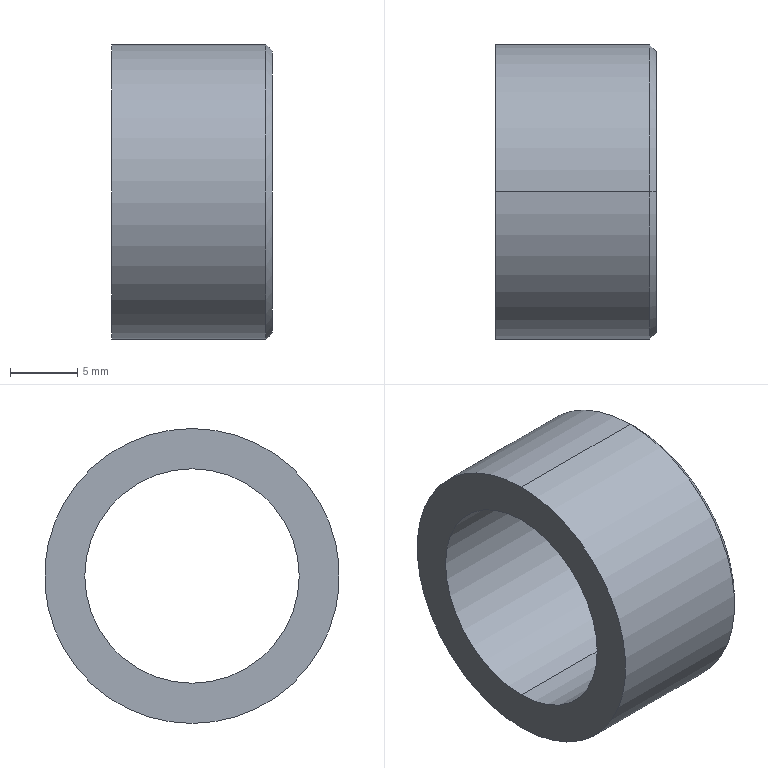Part | STEP file | Guide wheel mechanism revised.sldasm-Part-41 | 1 solid | 10 faces | box 12 x 22 x 22 mm | volume 2134 mm3 | cone 4 | cylinder 4 | plane 2 | commonest cylinder face diameters 16 x2 22 x2
STEP:
#1=CARTESIAN_POINT('',(11.5,0.,8.));
#2=VERTEX_POINT('',#1);
#3=CARTESIAN_POINT('',(11.5,0.,-8.));
#4=VERTEX_POINT('',#3);
#5=CARTESIAN_POINT('',(11.5,0.,0.));
#6=DIRECTION('',(1.,0.,0.));
#7=DIRECTION('',(0.,0.,1.));
#8=AXIS2_PLACEMENT_3D('',#5,#6,#7);
#9=CIRCLE('',#8,8.);
#10=EDGE_CURVE('',#2,#4,#9,.T.);
#11=ORIENTED_EDGE('',*,*,#10,.F.);
#12=CARTESIAN_POINT('',(12.,0.,8.5));
#13=VERTEX_POINT('',#12);
#14=CARTESIAN_POINT('',(12.,0.,8.5));
#15=DIRECTION('',(0.7071,0.,0.7071));
#16=VECTOR('',#15,1000.);
#17=LINE('',#14,#16);
#18=EDGE_CURVE('',#2,#13,#17,.T.);
#19=ORIENTED_EDGE('',*,*,#18,.T.);
#20=CARTESIAN_POINT('',(12.,0.,-8.5));
#21=VERTEX_POINT('',#20);
#22=CARTESIAN_POINT('',(12.,0.,0.));
#23=DIRECTION('',(-1.,0.,0.));
#24=DIRECTION('',(0.,0.,1.));
#25=AXIS2_PLACEMENT_3D('',#22,#23,#24);
#26=CIRCLE('',#25,8.5);
#27=EDGE_CURVE('',#21,#13,#26,.T.);
#28=ORIENTED_EDGE('',*,*,#27,.F.);
#29=CARTESIAN_POINT('',(12.,0.,-8.5));
#30=DIRECTION('',(0.7071,0.,-0.7071));
#31=VECTOR('',#30,1000.);
#32=LINE('',#29,#31);
#33=EDGE_CURVE('',#4,#21,#32,.T.);
#34=ORIENTED_EDGE('',*,*,#33,.F.);
#35=EDGE_LOOP('',(#11,#19,#28,#34));
#36=FACE_OUTER_BOUND('',#35,.T.);
#37=CARTESIAN_POINT('',(12.,0.,0.));
#38=DIRECTION('',(1.,0.,0.));
#39=DIRECTION('',(0.,0.,-1.));
#40=AXIS2_PLACEMENT_3D('',#37,#38,#39);
#41=CONICAL_SURFACE('',#40,8.5,0.7854);
#42=ADVANCED_FACE('',(#36),#41,.F.);
#43=CARTESIAN_POINT('',(12.,0.,-10.5));
#44=VERTEX_POINT('',#43);
#45=CARTESIAN_POINT('',(12.,0.,10.5));
#46=VERTEX_POINT('',#45);
#47=CARTESIAN_POINT('',(12.,0.,0.));
#48=DIRECTION('',(1.,0.,0.));
#49=DIRECTION('',(0.,0.,1.));
#50=AXIS2_PLACEMENT_3D('',#47,#48,#49);
#51=CIRCLE('',#50,10.5);
#52=EDGE_CURVE('',#44,#46,#51,.T.);
#53=ORIENTED_EDGE('',*,*,#52,.F.);
#54=CARTESIAN_POINT('',(11.5,0.,-11.));
#55=VERTEX_POINT('',#54);
#56=CARTESIAN_POINT('',(11.5,0.,-11.));
#57=DIRECTION('',(-0.7071,0.,-0.7071));
#58=VECTOR('',#57,1000.);
#59=LINE('',#56,#58);
#60=EDGE_CURVE('',#44,#55,#59,.T.);
#61=ORIENTED_EDGE('',*,*,#60,.T.);
#62=CARTESIAN_POINT('',(11.5,0.,11.));
#63=VERTEX_POINT('',#62);
#64=CARTESIAN_POINT('',(11.5,0.,0.));
#65=DIRECTION('',(-1.,0.,0.));
#66=DIRECTION('',(0.,0.,1.));
#67=AXIS2_PLACEMENT_3D('',#64,#65,#66);
#68=CIRCLE('',#67,11.);
#69=EDGE_CURVE('',#63,#55,#68,.T.);
#70=ORIENTED_EDGE('',*,*,#69,.F.);
#71=CARTESIAN_POINT('',(11.5,0.,11.));
#72=DIRECTION('',(-0.7071,0.,0.7071));
#73=VECTOR('',#72,1000.);
#74=LINE('',#71,#73);
#75=EDGE_CURVE('',#46,#63,#74,.T.);
#76=ORIENTED_EDGE('',*,*,#75,.F.);
#77=EDGE_LOOP('',(#53,#61,#70,#76));
#78=FACE_OUTER_BOUND('',#77,.T.);
#79=CARTESIAN_POINT('',(11.5,0.,0.));
#80=DIRECTION('',(-1.,0.,0.));
#81=DIRECTION('',(0.,0.,1.));
#82=AXIS2_PLACEMENT_3D('',#79,#80,#81);
#83=CONICAL_SURFACE('',#82,11.,0.7854);
#84=ADVANCED_FACE('',(#78),#83,.T.);
#85=ORIENTED_EDGE('',*,*,#69,.T.);
#86=CARTESIAN_POINT('',(0.,0.,-11.));
#87=VERTEX_POINT('',#86);
#88=CARTESIAN_POINT('',(12.,0.,-11.));
#89=DIRECTION('',(-1.,0.,0.));
#90=VECTOR('',#89,1000.);
#91=LINE('',#88,#90);
#92=EDGE_CURVE('',#55,#87,#91,.T.);
#93=ORIENTED_EDGE('',*,*,#92,.T.);
#94=CARTESIAN_POINT('',(0.,0.,11.));
#95=VERTEX_POINT('',#94);
#96=CARTESIAN_POINT('',(0.,0.,0.));
#97=DIRECTION('',(-1.,0.,0.));
#98=DIRECTION('',(0.,0.,1.));
#99=AXIS2_PLACEMENT_3D('',#96,#97,#98);
#100=CIRCLE('',#99,11.);
#101=EDGE_CURVE('',#95,#87,#100,.T.);
#102=ORIENTED_EDGE('',*,*,#101,.F.);
#103=CARTESIAN_POINT('',(12.,0.,11.));
#104=DIRECTION('',(-1.,0.,0.));
#105=VECTOR('',#104,1000.);
#106=LINE('',#103,#105);
#107=EDGE_CURVE('',#63,#95,#106,.T.);
#108=ORIENTED_EDGE('',*,*,#107,.F.);
#109=EDGE_LOOP('',(#85,#93,#102,#108));
#110=FACE_OUTER_BOUND('',#109,.T.);
#111=CARTESIAN_POINT('',(12.,0.,0.));
#112=DIRECTION('',(-1.,0.,0.));
#113=DIRECTION('',(0.,0.,1.));
#114=AXIS2_PLACEMENT_3D('',#111,#112,#113);
#115=CYLINDRICAL_SURFACE('',#114,11.);
#116=ADVANCED_FACE('',(#110),#115,.T.);
#117=ORIENTED_EDGE('',*,*,#10,.T.);
#118=CARTESIAN_POINT('',(0.,0.,-8.));
#119=VERTEX_POINT('',#118);
#120=CARTESIAN_POINT('',(12.,0.,-8.));
#121=DIRECTION('',(-1.,0.,0.));
#122=VECTOR('',#121,1000.);
#123=LINE('',#120,#122);
#124=EDGE_CURVE('',#4,#119,#123,.T.);
#125=ORIENTED_EDGE('',*,*,#124,.T.);
#126=CARTESIAN_POINT('',(0.,0.,8.));
#127=VERTEX_POINT('',#126);
#128=CARTESIAN_POINT('',(0.,0.,0.));
#129=DIRECTION('',(-1.,0.,0.));
#130=DIRECTION('',(0.,0.,1.));
#131=AXIS2_PLACEMENT_3D('',#128,#129,#130);
#132=CIRCLE('',#131,8.);
#133=EDGE_CURVE('',#119,#127,#132,.T.);
#134=ORIENTED_EDGE('',*,*,#133,.T.);
#135=CARTESIAN_POINT('',(12.,0.,8.));
#136=DIRECTION('',(-1.,0.,0.));
#137=VECTOR('',#136,1000.);
#138=LINE('',#135,#137);
#139=EDGE_CURVE('',#2,#127,#138,.T.);
#140=ORIENTED_EDGE('',*,*,#139,.F.);
#141=EDGE_LOOP('',(#117,#125,#134,#140));
#142=FACE_OUTER_BOUND('',#141,.T.);
#143=CARTESIAN_POINT('',(12.,0.,0.));
#144=DIRECTION('',(-1.,0.,0.));
#145=DIRECTION('',(0.,0.,1.));
#146=AXIS2_PLACEMENT_3D('',#143,#144,#145);
#147=CYLINDRICAL_SURFACE('',#146,8.);
#148=ADVANCED_FACE('',(#142),#147,.F.);
#149=ORIENTED_EDGE('',*,*,#124,.F.);
#150=CARTESIAN_POINT('',(11.5,0.,0.));
#151=DIRECTION('',(1.,0.,0.));
#152=DIRECTION('',(0.,0.,1.));
#153=AXIS2_PLACEMENT_3D('',#150,#151,#152);
#154=CIRCLE('',#153,8.);
#155=EDGE_CURVE('',#4,#2,#154,.T.);
#156=ORIENTED_EDGE('',*,*,#155,.T.);
#157=ORIENTED_EDGE('',*,*,#139,.T.);
#158=CARTESIAN_POINT('',(0.,0.,0.));
#159=DIRECTION('',(-1.,0.,0.));
#160=DIRECTION('',(0.,0.,1.));
#161=AXIS2_PLACEMENT_3D('',#158,#159,#160);
#162=CIRCLE('',#161,8.);
#163=EDGE_CURVE('',#127,#119,#162,.T.);
#164=ORIENTED_EDGE('',*,*,#163,.T.);
#165=EDGE_LOOP('',(#149,#156,#157,#164));
#166=FACE_OUTER_BOUND('',#165,.T.);
#167=CARTESIAN_POINT('',(12.,0.,0.));
#168=DIRECTION('',(-1.,0.,0.));
#169=DIRECTION('',(0.,0.,1.));
#170=AXIS2_PLACEMENT_3D('',#167,#168,#169);
#171=CYLINDRICAL_SURFACE('',#170,8.);
#172=ADVANCED_FACE('',(#166),#171,.F.);
#173=ORIENTED_EDGE('',*,*,#27,.T.);
#174=CARTESIAN_POINT('',(12.,0.,0.));
#175=DIRECTION('',(-1.,0.,0.));
#176=DIRECTION('',(0.,0.,1.));
#177=AXIS2_PLACEMENT_3D('',#174,#175,#176);
#178=CIRCLE('',#177,8.5);
#179=EDGE_CURVE('',#13,#21,#178,.T.);
#180=ORIENTED_EDGE('',*,*,#179,.T.);
#181=EDGE_LOOP('',(#173,#180));
#182=FACE_BOUND('',#181,.T.);
#183=CARTESIAN_POINT('',(12.,0.,0.));
#184=DIRECTION('',(1.,0.,0.));
#185=DIRECTION('',(0.,0.,1.));
#186=AXIS2_PLACEMENT_3D('',#183,#184,#185);
#187=CIRCLE('',#186,10.5);
#188=EDGE_CURVE('',#46,#44,#187,.T.);
#189=ORIENTED_EDGE('',*,*,#188,.T.);
#190=ORIENTED_EDGE('',*,*,#52,.T.);
#191=EDGE_LOOP('',(#189,#190));
#192=FACE_OUTER_BOUND('',#191,.T.);
#193=CARTESIAN_POINT('',(12.,9.,0.));
#194=DIRECTION('',(-1.,0.,0.));
#195=DIRECTION('',(0.,0.,1.));
#196=AXIS2_PLACEMENT_3D('',#193,#194,#195);
#197=PLANE('',#196);
#198=ADVANCED_FACE('',(#182,#192),#197,.F.);
#199=ORIENTED_EDGE('',*,*,#163,.F.);
#200=ORIENTED_EDGE('',*,*,#133,.F.);
#201=EDGE_LOOP('',(#199,#200));
#202=FACE_BOUND('',#201,.T.);
#203=ORIENTED_EDGE('',*,*,#101,.T.);
#204=CARTESIAN_POINT('',(0.,0.,0.));
#205=DIRECTION('',(-1.,0.,0.));
#206=DIRECTION('',(0.,0.,1.));
#207=AXIS2_PLACEMENT_3D('',#204,#205,#206);
#208=CIRCLE('',#207,11.);
#209=EDGE_CURVE('',#87,#95,#208,.T.);
#210=ORIENTED_EDGE('',*,*,#209,.T.);
#211=EDGE_LOOP('',(#203,#210));
#212=FACE_OUTER_BOUND('',#211,.T.);
#213=CARTESIAN_POINT('',(0.,10.,0.));
#214=DIRECTION('',(1.,0.,0.));
#215=DIRECTION('',(0.,0.,-1.));
#216=AXIS2_PLACEMENT_3D('',#213,#214,#215);
#217=PLANE('',#216);
#218=ADVANCED_FACE('',(#202,#212),#217,.F.);
#219=ORIENTED_EDGE('',*,*,#92,.F.);
#220=CARTESIAN_POINT('',(11.5,0.,0.));
#221=DIRECTION('',(-1.,0.,0.));
#222=DIRECTION('',(0.,0.,1.));
#223=AXIS2_PLACEMENT_3D('',#220,#221,#222);
#224=CIRCLE('',#223,11.);
#225=EDGE_CURVE('',#55,#63,#224,.T.);
#226=ORIENTED_EDGE('',*,*,#225,.T.);
#227=ORIENTED_EDGE('',*,*,#107,.T.);
#228=ORIENTED_EDGE('',*,*,#209,.F.);
#229=EDGE_LOOP('',(#219,#226,#227,#228));
#230=FACE_OUTER_BOUND('',#229,.T.);
#231=CARTESIAN_POINT('',(12.,0.,0.));
#232=DIRECTION('',(-1.,0.,0.));
#233=DIRECTION('',(0.,0.,1.));
#234=AXIS2_PLACEMENT_3D('',#231,#232,#233);
#235=CYLINDRICAL_SURFACE('',#234,11.);
#236=ADVANCED_FACE('',(#230),#235,.T.);
#237=ORIENTED_EDGE('',*,*,#60,.F.);
#238=ORIENTED_EDGE('',*,*,#188,.F.);
#239=ORIENTED_EDGE('',*,*,#75,.T.);
#240=ORIENTED_EDGE('',*,*,#225,.F.);
#241=EDGE_LOOP('',(#237,#238,#239,#240));
#242=FACE_OUTER_BOUND('',#241,.T.);
#243=CARTESIAN_POINT('',(11.5,0.,0.));
#244=DIRECTION('',(-1.,0.,0.));
#245=DIRECTION('',(0.,0.,1.));
#246=AXIS2_PLACEMENT_3D('',#243,#244,#245);
#247=CONICAL_SURFACE('',#246,11.,0.7854);
#248=ADVANCED_FACE('',(#242),#247,.T.);
#249=ORIENTED_EDGE('',*,*,#18,.F.);
#250=ORIENTED_EDGE('',*,*,#155,.F.);
#251=ORIENTED_EDGE('',*,*,#33,.T.);
#252=ORIENTED_EDGE('',*,*,#179,.F.);
#253=EDGE_LOOP('',(#249,#250,#251,#252));
#254=FACE_OUTER_BOUND('',#253,.T.);
#255=CARTESIAN_POINT('',(12.,0.,0.));
#256=DIRECTION('',(1.,0.,0.));
#257=DIRECTION('',(0.,0.,-1.));
#258=AXIS2_PLACEMENT_3D('',#255,#256,#257);
#259=CONICAL_SURFACE('',#258,8.5,0.7854);
#260=ADVANCED_FACE('',(#254),#259,.F.);
#261=CLOSED_SHELL('',(#42,#84,#116,#148,#172,#198,#218,#236,#248,#260));
#262=MANIFOLD_SOLID_BREP('',#261);
#263=CARTESIAN_POINT('',(0.,0.,0.));
#264=DIRECTION('',(0.,0.,1.));
#265=DIRECTION('',(1.,0.,0.));
#266=AXIS2_PLACEMENT_3D('',#263,#264,#265);
#267=(LENGTH_UNIT()NAMED_UNIT(*)SI_UNIT(.MILLI.,.METRE.));
#268=UNCERTAINTY_MEASURE_WITH_UNIT(LENGTH_MEASURE(0.00001),#267,'','');
#269=(NAMED_UNIT(*)PLANE_ANGLE_UNIT()SI_UNIT($,.RADIAN.));
#270=(NAMED_UNIT(*)SI_UNIT($,.STERADIAN.)SOLID_ANGLE_UNIT());
#271=(GEOMETRIC_REPRESENTATION_CONTEXT(3)GLOBAL_UNCERTAINTY_ASSIGNED_CONTEXT((#268))GLOBAL_UNIT_ASSIGNED_CONTEXT((#267,#269,#270))REPRESENTATION_CONTEXT('',''));
#272=ADVANCED_BREP_SHAPE_REPRESENTATION('',(#262,#266),#271);